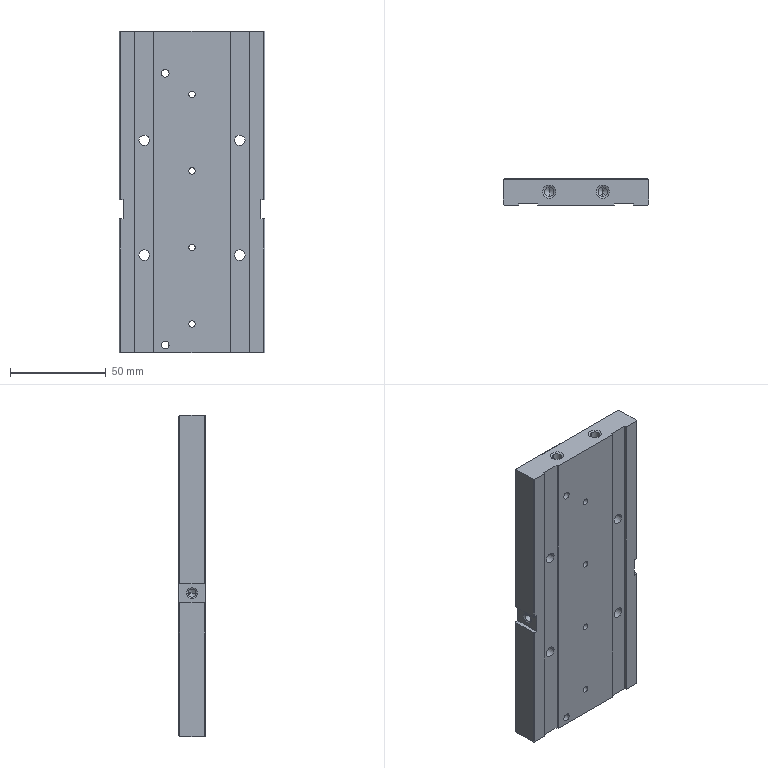Part | NX | 1 solid | 104 faces | box 76 x 14 x 168 mm | volume 170208 mm3 | plane 36 | cylinder 36 | cone 32 | commonest cylinder face diameters 3.3 x8 5.5 x8 10 x8 4 x4 4.2 x4 5 x4